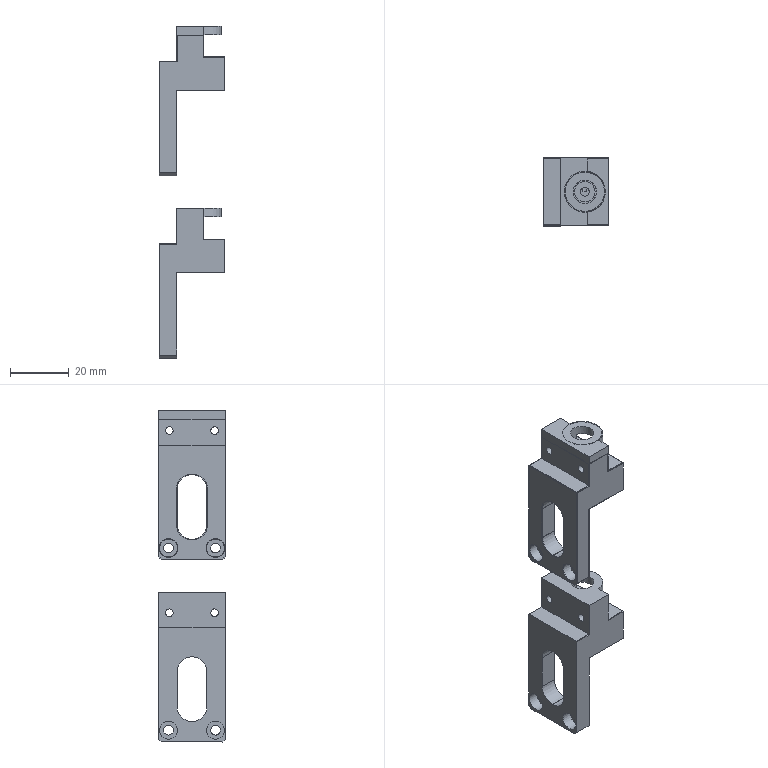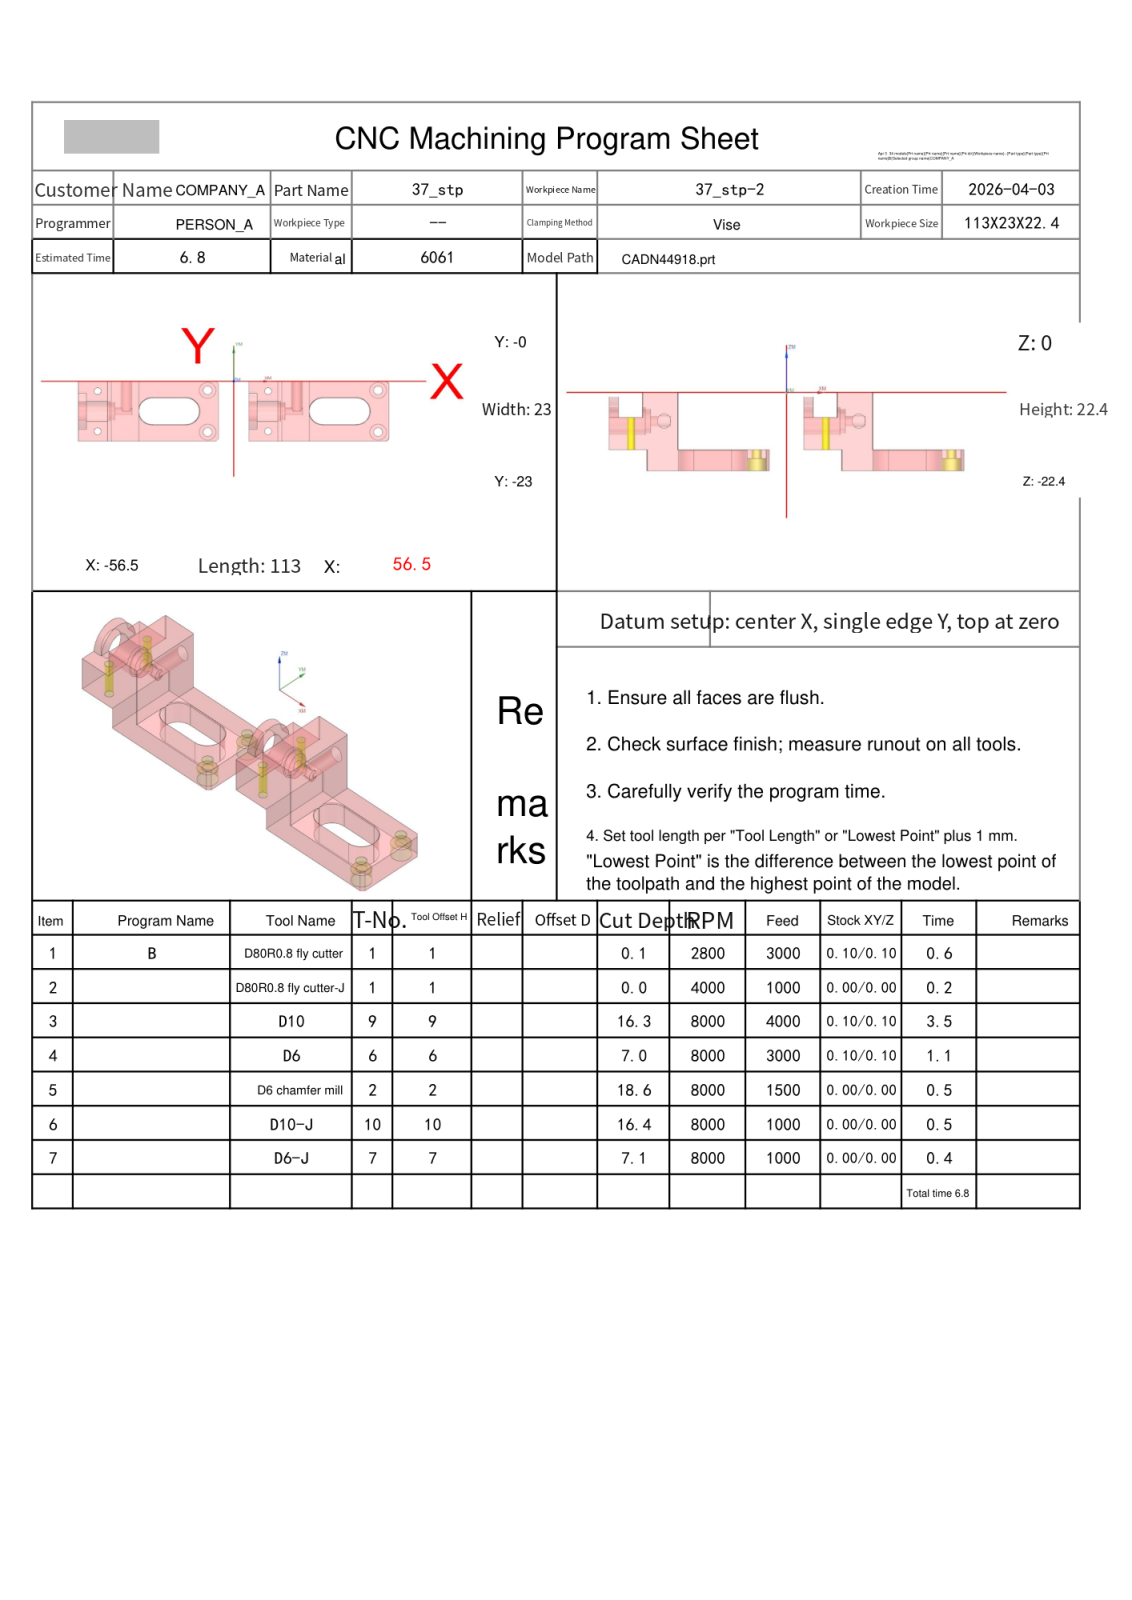NC program | NX | posted by the shop | part box 22.4 x 23 x 113 mm
Lines 3244 to 3535 of 3535:
N6 T10 M06
(D10-J  D=10. R=0. H=10 ce=0.40 di=0.00)
G00 G90 G54 X-19.3 Y7. M03 S8000
G43 H10 Z12.4
M08
Z-14.9
G01 Z-16.4 F1000.
Y3.
G03 X-17.3 Y1. I2. J0.0
G01 X-6.498
G02 X-5.794 Y.708 I-.002 J-1.
G01 X-4.792 Y-.294
G02 X-4.5 Y-.998 I-.708 J-.706
G01 Y-22.002
G02 X-4.792 Y-22.706 I-1. J.002
G01 X-5.794 Y-23.708
G02 X-6.498 Y-24. I-.706 J.708
G01 X-28.102
G02 X-29.1 Y-23.002 I.002 J1.
G01 Y-16.798
G02 X-28.102 Y-15.8 I1. J-.002
G01 X-17.5
G03 X-14.403 Y-14.437 I0.0 J4.2
G02 X-13.665 Y-14.112 I.737 J-.675
X-12.942 Y-14.422 I0.0 J-1.
G01 X-9.891 Y-17.619
X-9.828 Y-17.695
X-9.749 Y-17.752
G02 X-9.5 Y-18.288 I-.451 J-.535
G01 Y-18.302
G02 X-10.2 Y-19. I-.7 J.002
G01 X-10.213
G02 X-10.912 Y-18.3 I.002 J.7
G01 Y-18.294
Y-18.287
G03 X-11.422 Y-17.437 I-.963 J0.0
G01 X-14.135 Y-15.995
G02 X-14.665 Y-15.112 I.47 J.883
X-14.403 Y-14.437 I1. J0.0
G03 X-13.3 Y-11.6 I-3.097 J2.836
G01 Y-11.4
G03 X-17.5 Y-7.2 I-4.2 J0.0
G01 X-28.102
G02 X-29.1 Y-6.202 I.002 J1.
G01 Y.002
G02 X-28.102 Y1. I1. J-.002
G01 X-12.3
G02 X-11.334 Y.258 I0.0 J-1.
G01 X-10.482 Y-2.936
G03 X-9.726 Y-4.184 I2.522 J.673
G02 X-9.5 Y-4.7 I-.474 J-.516
G01 Y-4.714
G02 X-10.2 Y-5.413 I-.7 J.002
X-10.728 Y-5.173 I0.0 J.7
X-10.912 Y-4.7 I.516 J.473
X-10.452 Y-4.043 I.7 J0.0
X-10.211 Y-4. I.241 J-.657
G01 X-10.198
G02 X-9.589 Y-4.358 I-.002 J-.7
G03 X-7.844 Y-5.382 I1.745 J.976
X-6.867 Y-5.127 I0.0 J2.
G01 Z-14.9
G00 Z12.4
X42.7 Y7.
Z-14.9
G01 Z-16.4
Y3.
G03 X44.7 Y1. I2. J0.0
G01 X55.502
G02 X56.206 Y.708 I-.002 J-1.
G01 X57.208 Y-.294
G02 X57.5 Y-.998 I-.708 J-.706
G01 Y-22.002
G02 X57.208 Y-22.706 I-1. J.002
G01 X56.206 Y-23.708
G02 X55.502 Y-24. I-.706 J.708
G01 X33.898
G02 X32.9 Y-23.002 I.002 J1.
G01 Y-16.798
G02 X33.898 Y-15.8 I1. J-.002
G01 X44.5
G03 X47.597 Y-14.437 I0.0 J4.2
G02 X48.335 Y-14.112 I.737 J-.675
X49.058 Y-14.422 I0.0 J-1.
G01 X52.109 Y-17.619
X52.171 Y-17.695
X52.251 Y-17.752
G02 X52.5 Y-18.288 I-.451 J-.535
G01 Y-18.302
G02 X51.8 Y-19. I-.7 J.002
G01 X51.787
G02 X51.088 Y-18.3 I.002 J.7
G01 Y-18.294
Y-18.287
G03 X50.578 Y-17.437 I-.963 J0.0
G01 X47.865 Y-15.995
G02 X47.335 Y-15.112 I.47 J.883
X47.597 Y-14.437 I1. J0.0
G03 X48.7 Y-11.6 I-3.097 J2.837
G01 Y-11.4
G03 X44.5 Y-7.2 I-4.2 J0.0
G01 X33.898
G02 X32.9 Y-6.202 I.002 J1.
G01 Y.002
G02 X33.898 Y1. I1. J-.002
G01 X49.7
G02 X50.666 Y.258 I0.0 J-1.
G01 X51.518 Y-2.935
G03 X52.274 Y-4.184 I2.522 J.673
G02 X52.5 Y-4.7 I-.474 J-.516
G01 Y-4.714
G02 X51.8 Y-5.413 I-.7 J.002
X51.272 Y-5.173 I0.0 J.7
X51.088 Y-4.7 I.516 J.473
X51.548 Y-4.043 I.7 J0.0
X51.789 Y-4. I.241 J-.657
G01 X51.802
G02 X52.411 Y-4.358 I-.002 J-.7
G03 X54.156 Y-5.382 I1.745 J.976
X55.133 Y-5.127 I0.0 J2.
G01 X63.5
Z-14.9
G00 Z12.4
G00 G90 X28.932 Y7.191 M03 S8000
Z12.4
Z-15.4
G01 Z-16.4 F1000.
G41 D10
X28.873 Y7.
G03 X28.785 Y6.414 I1.912 J-.586
X29.371 Y5. I2. J0.0
G01 X32.5 Y1.871
Y-11.2
G03 X34.5 Y-13.2 I2. J0.0
G01 G40 X34.7
Z-15.4
G00 Y-9.8
G01 Z-16.4
G41 D10
X34.5
G03 X32.5 Y-11.8 I0.0 J-2.
G01 Y-24.871
X29.371 Y-28.
G03 X28.785 Y-29.414 I1.414 J-1.414
X28.873 Y-30. I2. J0.0
G01 G40 X28.932 Y-30.191
Z-15.4
G00 Z12.4
X-27.3 Y-9.8
Z-15.4
G01 Z-16.4
G41 D10
X-27.5
G03 X-29.5 Y-11.8 I0.0 J-2.
G01 Y-24.871
X-32.629 Y-28.
G03 X-33.215 Y-29.414 I1.414 J-1.414
X-33.127 Y-30. I2. J0.0
G01 G40 X-33.068 Y-30.191
Z-15.4
G00 Z12.4
Y7.191
Z-15.4
G01 Z-16.4
G41 D10
X-33.127 Y7.
G03 X-33.215 Y6.414 I1.912 J-.586
X-32.629 Y5. I2. J0.0
G01 X-29.5 Y1.871
Y-11.2
G03 X-27.5 Y-13.2 I2. J0.0
G01 G40 X-27.3
Z-15.4
G00 Z12.4
G91 G28 Z0.0
M05
M09
G91 G28 Z0.0
M01
N7 T07 M06
(D6-J  D=6. R=0. H=07 ce=0.40 di=0.00)
G00 G90 G54 X-54.425 Y4.2 M03 S8000
G43 H07 Z12.4
M08
Z-5.65
G01 Z-7.15 F1000.
Y1.8
G03 X-53.225 Y.6 I1.2 J0.0
G01 X-49.949
G02 X-49.35 Y.001 I-.001 J-.6
G01 Y-23.001
G02 X-49.949 Y-23.6 I-.6 J.001
G01 X-56.501
G02 X-57.1 Y-23.001 I.001 J.6
G01 Y-22.419
G02 X-56.501 Y-21.821 I.6 J-.001
G01 X-50.1
Y-1.179
X-56.501
G02 X-57.1 Y-.581 I.001 J.6
G01 Y.001
G02 X-56.501 Y.6 I.6 J-.001
G01 X-53.225
X-52.225
G03 X-51.025 Y1.8 I0.0 J1.2
G01 Y4.2
Z-5.65
G00 Z-3.15
X7.575
Z-5.65
G01 Z-7.15
Y1.8
G03 X8.775 Y.6 I1.2 J0.0
G01 X12.051
G02 X12.65 Y.001 I-.001 J-.6
G01 Y-23.001
G02 X12.051 Y-23.6 I-.6 J.001
G01 X5.499
G02 X4.9 Y-23.001 I.001 J.6
G01 Y-22.419
G02 X5.499 Y-21.821 I.6 J-.001
G01 X11.9
Y-1.179
X5.499
G02 X4.9 Y-.581 I.001 J.6
G01 Y.001
G02 X5.499 Y.6 I.6 J-.001
G01 X8.775
X9.775
G03 X10.975 Y1.8 I0.0 J1.2
G01 Y4.2
Z-5.65
G00 Z12.4
G00 G90 X-46.752 Y-27.391 M03 S8000
Z12.4
Z-6.15
G01 Z-7.15 F1000.
G41 D07
X-46.694 Y-27.2
G03 X-46.641 Y-26.849 I-1.147 J.351
X-46.993 Y-26. I-1.2 J0.0
G01 X-48.95 Y-24.043
Y1.043
X-46.993 Y3.
G03 X-46.641 Y3.849 I-.849 J.849
X-46.694 Y4.2 I-1.2 J0.0
G01 G40 X-46.752 Y4.391
Z-6.15
G00 X-60.7 Y-.18
G01 Z-7.15
G41 D07
Y-.38
G03 X-59.5 Y-1.579 I1.2 J0.0
G01 X-50.5
Y-21.421
X-59.5
G03 X-60.7 Y-22.621 I0.0 J-1.2
G01 G40 Y-22.821
Z-6.15
G00 Z12.4
X1.3 Y-.18
Z-6.15
G01 Z-7.15
G41 D07
Y-.38
G03 X2.5 Y-1.579 I1.2 J0.0
G01 X11.5
Y-21.421
X2.5
G03 X1.3 Y-22.621 I0.0 J-1.2
G01 G40 Y-22.821
Z-6.15
G00 X15.248 Y-27.391
G01 Z-7.15
G41 D07
X15.306 Y-27.2
G03 X15.359 Y-26.849 I-1.147 J.351
X15.007 Y-26. I-1.2 J0.0
G01 X13.05 Y-24.043
Y1.043
X15.007 Y3.
G03 X15.359 Y3.849 I-.849 J.849
X15.306 Y4.2 I-1.2 J0.0
G01 G40 X15.248 Y4.391
Z-6.15
G00 Z12.4
M05
M09
G91 G28 Z0.0
G91 G28 Y0.0
M30
%